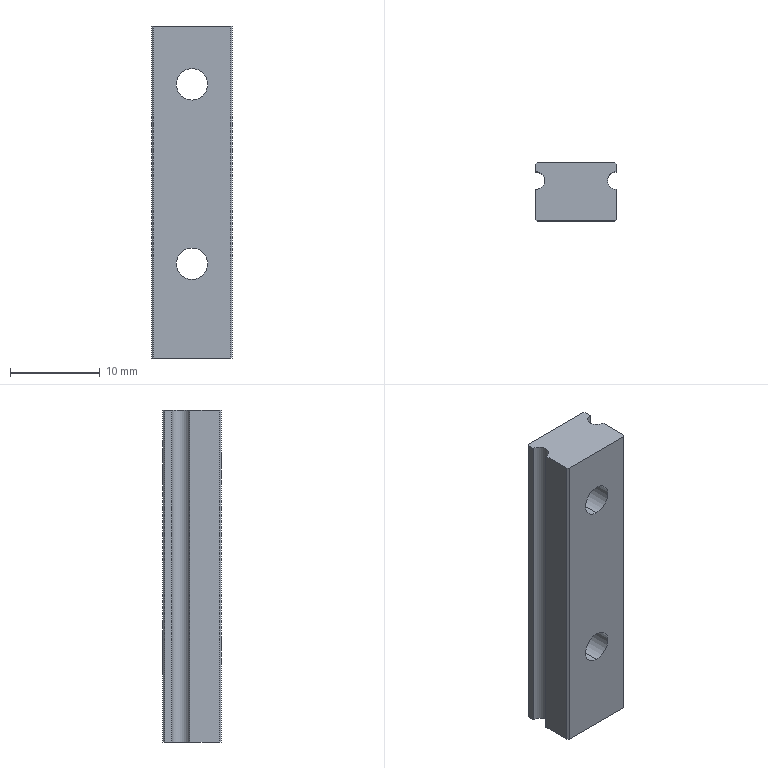Part | STEP file | rail-01 MGN9C1R-37-Z1CM_PERSON_A hot-press welding configuration | 1 solid | 25 faces | box 9 x 6.5 x 37 mm | volume 1790 mm3 | plane 14 | cylinder 11 | commonest cylinder face diameters 3.5 x4 6 x4 2 x3